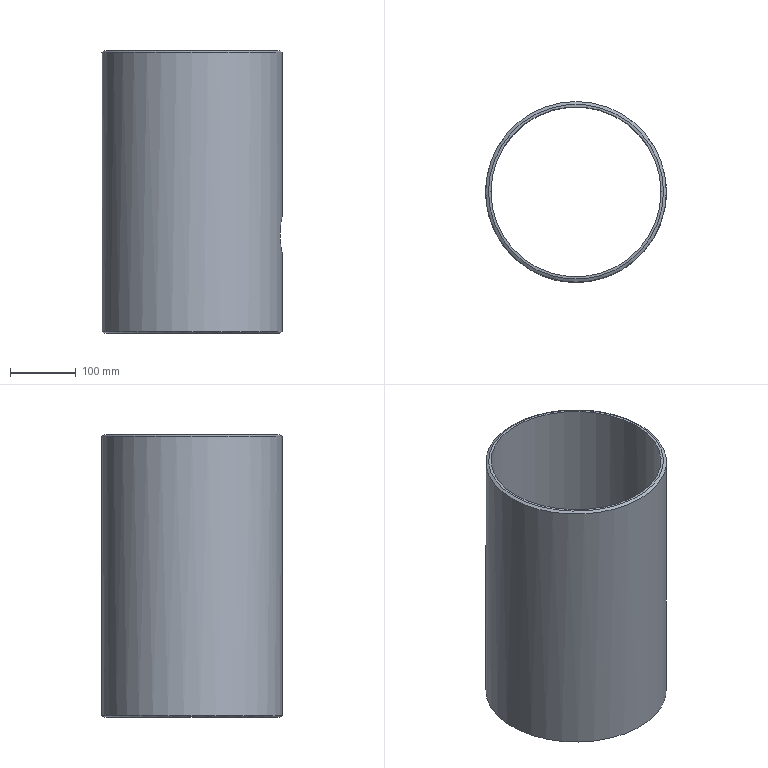Part | NX | features DATUM_CSYS 2, CHAMFER 1, CYLINDER 1, EXTRUDE 1, Resize Face 1, SHELL 1, SKETCH 1 | 1 solid | 7 faces | box 275 x 275 x 430 mm | volume 2853471 mm3 | cylinder 3 | plane 2 | cone 2 | commonest cylinder face diameters 60 x1 259 x1 275 x1
STEP:
#1=CARTESIAN_POINT('',(137.5,0.,2.5));
#2=VERTEX_POINT('',#1);
#3=CARTESIAN_POINT('',(0.,0.,2.5));
#4=DIRECTION('',(0.,0.,1.));
#5=DIRECTION('',(1.,0.,0.));
#6=AXIS2_PLACEMENT_3D('',#3,#4,#5);
#7=CIRCLE('',#6,137.5);
#8=EDGE_CURVE('',#2,#2,#7,.T.);
#9=ORIENTED_EDGE('',*,*,#8,.T.);
#10=EDGE_LOOP('',(#9));
#11=FACE_BOUND('',#10,.T.);
#12=CARTESIAN_POINT('',(-137.5,0.,427.5));
#13=VERTEX_POINT('',#12);
#14=CARTESIAN_POINT('',(0.,0.,427.5));
#15=DIRECTION('',(0.,0.,-1.));
#16=DIRECTION('',(-1.,0.,0.));
#17=AXIS2_PLACEMENT_3D('',#14,#15,#16);
#18=CIRCLE('',#17,137.5);
#19=EDGE_CURVE('',#13,#13,#18,.T.);
#20=ORIENTED_EDGE('',*,*,#19,.T.);
#21=EDGE_LOOP('',(#20));
#22=FACE_BOUND('',#21,.T.);
#23=CARTESIAN_POINT('',(137.5,0.,120.));
#24=VERTEX_POINT('',#23);
#25=CARTESIAN_POINT('',(137.14,11.856,121.591));
#26=CARTESIAN_POINT('',(137.679,-0.009269,119.207));
#27=CARTESIAN_POINT('',(137.143,-11.819,121.58));
#28=CARTESIAN_POINT('',(135.855,-21.765,128.245));
#29=CARTESIAN_POINT('',(134.555,-28.42,138.183));
#30=CARTESIAN_POINT('',(134.004,-30.786,149.979));
#31=CARTESIAN_POINT('',(134.552,-28.435,161.792));
#32=CARTESIAN_POINT('',(135.856,-21.764,171.76));
#33=CARTESIAN_POINT('',(137.143,-11.813,178.423));
#34=CARTESIAN_POINT('',(137.678,-0.01305,180.786));
#35=CARTESIAN_POINT('',(137.145,11.791,178.432));
#36=CARTESIAN_POINT('',(135.859,21.742,171.778));
#37=CARTESIAN_POINT('',(134.556,28.414,161.839));
#38=CARTESIAN_POINT('',(134.004,30.789,150.018));
#39=CARTESIAN_POINT('',(134.553,28.431,138.203));
#40=CARTESIAN_POINT('',(135.854,21.771,128.255));
#41=CARTESIAN_POINT('',(137.14,11.856,121.591));
#42=CARTESIAN_POINT('',(137.679,-0.009269,119.207));
#43=CARTESIAN_POINT('',(137.143,-11.819,121.58));
#44=B_SPLINE_CURVE_WITH_KNOTS('',3,(#25,#26,#27,#28,#29,#30,#31,#32,#33,#34,#35,#36,#37,#38,#39,#40,#41,#42,#43),.UNSPECIFIED.,.T.,.F.,(1,1,1,1,1,1,1,1,1,1,1,1,1,1,1,1,1,1,1,1,1,1,1),(-0.03527,-0.02352,-0.01176,0.,0.01176,0.02352,0.03527,0.04703,0.05879,0.07055,0.08231,0.09406,0.1058,0.1176,0.1293,0.1411,0.1529,0.1646,0.1764,0.1881,0.1999,0.2116,0.2234),.UNSPECIFIED.);
#45=EDGE_CURVE('',#24,#24,#44,.T.);
#46=ORIENTED_EDGE('',*,*,#45,.T.);
#47=EDGE_LOOP('',(#46));
#48=FACE_BOUND('',#47,.T.);
#49=CARTESIAN_POINT('',(0.,0.,0.));
#50=DIRECTION('',(0.,0.,1.));
#51=DIRECTION('',(1.,0.,0.));
#52=AXIS2_PLACEMENT_3D('',#49,#50,#51);
#53=CYLINDRICAL_SURFACE('',#52,137.5);
#54=ADVANCED_FACE('',(#11,#22,#48),#53,.T.);
#55=CARTESIAN_POINT('',(129.5,0.,430.));
#56=VERTEX_POINT('',#55);
#57=CARTESIAN_POINT('',(0.,0.,430.));
#58=DIRECTION('',(0.,0.,1.));
#59=DIRECTION('',(1.,0.,0.));
#60=AXIS2_PLACEMENT_3D('',#57,#58,#59);
#61=CIRCLE('',#60,129.5);
#62=EDGE_CURVE('',#56,#56,#61,.F.);
#63=ORIENTED_EDGE('',*,*,#62,.F.);
#64=EDGE_LOOP('',(#63));
#65=FACE_BOUND('',#64,.T.);
#66=CARTESIAN_POINT('',(-129.5,0.,0.));
#67=VERTEX_POINT('',#66);
#68=CARTESIAN_POINT('',(0.,0.,0.));
#69=DIRECTION('',(0.,0.,-1.));
#70=DIRECTION('',(-1.,0.,0.));
#71=AXIS2_PLACEMENT_3D('',#68,#69,#70);
#72=CIRCLE('',#71,129.5);
#73=EDGE_CURVE('',#67,#67,#72,.F.);
#74=ORIENTED_EDGE('',*,*,#73,.F.);
#75=EDGE_LOOP('',(#74));
#76=FACE_BOUND('',#75,.T.);
#77=CARTESIAN_POINT('',(129.5,0.,120.));
#78=VERTEX_POINT('',#77);
#79=CARTESIAN_POINT('',(129.118,11.859,121.593));
#80=CARTESIAN_POINT('',(129.691,-0.008952,119.206));
#81=CARTESIAN_POINT('',(129.12,-11.823,121.581));
#82=CARTESIAN_POINT('',(127.753,-21.765,128.246));
#83=CARTESIAN_POINT('',(126.369,-28.418,138.179));
#84=CARTESIAN_POINT('',(125.782,-30.787,149.978));
#85=CARTESIAN_POINT('',(126.366,-28.433,161.796));
#86=CARTESIAN_POINT('',(127.754,-21.762,171.761));
#87=CARTESIAN_POINT('',(129.121,-11.817,178.421));
#88=CARTESIAN_POINT('',(129.689,-0.01338,180.787));
#89=CARTESIAN_POINT('',(129.123,11.795,178.431));
#90=CARTESIAN_POINT('',(127.757,21.743,171.777));
#91=CARTESIAN_POINT('',(126.371,28.413,161.842));
#92=CARTESIAN_POINT('',(125.781,30.79,150.017));
#93=CARTESIAN_POINT('',(126.367,28.429,138.198));
#94=CARTESIAN_POINT('',(127.751,21.77,128.255));
#95=CARTESIAN_POINT('',(129.118,11.859,121.593));
#96=CARTESIAN_POINT('',(129.691,-0.008952,119.206));
#97=CARTESIAN_POINT('',(129.12,-11.823,121.581));
#98=B_SPLINE_CURVE_WITH_KNOTS('',3,(#79,#80,#81,#82,#83,#84,#85,#86,#87,#88,#89,#90,#91,#92,#93,#94,#95,#96,#97),.UNSPECIFIED.,.T.,.F.,(1,1,1,1,1,1,1,1,1,1,1,1,1,1,1,1,1,1,1,1,1,1,1),(-0.03529,-0.02353,-0.01176,0.,0.01176,0.02353,0.03529,0.04705,0.05881,0.07058,0.08234,0.0941,0.1059,0.1176,0.1294,0.1412,0.1529,0.1647,0.1764,0.1882,0.2,0.2117,0.2235),.UNSPECIFIED.);
#99=EDGE_CURVE('',#78,#78,#98,.T.);
#100=ORIENTED_EDGE('',*,*,#99,.F.);
#101=EDGE_LOOP('',(#100));
#102=FACE_BOUND('',#101,.T.);
#103=CARTESIAN_POINT('',(0.,0.,0.));
#104=DIRECTION('',(0.,0.,1.));
#105=DIRECTION('',(1.,0.,0.));
#106=AXIS2_PLACEMENT_3D('',#103,#104,#105);
#107=CYLINDRICAL_SURFACE('',#106,129.5);
#108=ADVANCED_FACE('',(#65,#76,#102),#107,.F.);
#109=CARTESIAN_POINT('',(133.17,0.,430.));
#110=VERTEX_POINT('',#109);
#111=CARTESIAN_POINT('',(0.,0.,430.));
#112=DIRECTION('',(0.,0.,1.));
#113=DIRECTION('',(1.,0.,0.));
#114=AXIS2_PLACEMENT_3D('',#111,#112,#113);
#115=CIRCLE('',#114,133.17);
#116=EDGE_CURVE('',#110,#110,#115,.T.);
#117=ORIENTED_EDGE('',*,*,#116,.T.);
#118=EDGE_LOOP('',(#117));
#119=FACE_BOUND('',#118,.T.);
#120=ORIENTED_EDGE('',*,*,#62,.T.);
#121=EDGE_LOOP('',(#120));
#122=FACE_BOUND('',#121,.T.);
#123=CARTESIAN_POINT('',(0.,0.,430.));
#124=DIRECTION('',(0.,0.,1.));
#125=DIRECTION('',(1.,0.,0.));
#126=AXIS2_PLACEMENT_3D('',#123,#124,#125);
#127=PLANE('',#126);
#128=ADVANCED_FACE('',(#119,#122),#127,.T.);
#129=CARTESIAN_POINT('',(-133.17,0.,0.));
#130=VERTEX_POINT('',#129);
#131=CARTESIAN_POINT('',(0.,0.,0.));
#132=DIRECTION('',(0.,0.,-1.));
#133=DIRECTION('',(-1.,0.,0.));
#134=AXIS2_PLACEMENT_3D('',#131,#132,#133);
#135=CIRCLE('',#134,133.17);
#136=EDGE_CURVE('',#130,#130,#135,.T.);
#137=ORIENTED_EDGE('',*,*,#136,.T.);
#138=EDGE_LOOP('',(#137));
#139=FACE_BOUND('',#138,.T.);
#140=ORIENTED_EDGE('',*,*,#73,.T.);
#141=EDGE_LOOP('',(#140));
#142=FACE_BOUND('',#141,.T.);
#143=CARTESIAN_POINT('',(0.,0.,0.));
#144=DIRECTION('',(0.,0.,-1.));
#145=DIRECTION('',(-1.,0.,0.));
#146=AXIS2_PLACEMENT_3D('',#143,#144,#145);
#147=PLANE('',#146);
#148=ADVANCED_FACE('',(#139,#142),#147,.T.);
#149=ORIENTED_EDGE('',*,*,#116,.F.);
#150=EDGE_LOOP('',(#149));
#151=FACE_BOUND('',#150,.T.);
#152=ORIENTED_EDGE('',*,*,#19,.F.);
#153=EDGE_LOOP('',(#152));
#154=FACE_BOUND('',#153,.T.);
#155=CARTESIAN_POINT('',(0.,0.,427.5));
#156=DIRECTION('',(0.,0.,-1.));
#157=DIRECTION('',(-1.,0.,0.));
#158=AXIS2_PLACEMENT_3D('',#155,#156,#157);
#159=CONICAL_SURFACE('',#158,137.5,1.047);
#160=ADVANCED_FACE('',(#151,#154),#159,.T.);
#161=ORIENTED_EDGE('',*,*,#136,.F.);
#162=EDGE_LOOP('',(#161));
#163=FACE_BOUND('',#162,.T.);
#164=ORIENTED_EDGE('',*,*,#8,.F.);
#165=EDGE_LOOP('',(#164));
#166=FACE_BOUND('',#165,.T.);
#167=CARTESIAN_POINT('',(0.,0.,2.5));
#168=DIRECTION('',(0.,0.,1.));
#169=DIRECTION('',(1.,0.,0.));
#170=AXIS2_PLACEMENT_3D('',#167,#168,#169);
#171=CONICAL_SURFACE('',#170,137.5,1.047);
#172=ADVANCED_FACE('',(#163,#166),#171,.T.);
#173=ORIENTED_EDGE('',*,*,#45,.F.);
#174=EDGE_LOOP('',(#173));
#175=FACE_BOUND('',#174,.T.);
#176=ORIENTED_EDGE('',*,*,#99,.T.);
#177=EDGE_LOOP('',(#176));
#178=FACE_BOUND('',#177,.T.);
#179=CARTESIAN_POINT('',(720.,0.,150.));
#180=DIRECTION('',(-1.,0.,0.));
#181=DIRECTION('',(0.,0.,1.));
#182=AXIS2_PLACEMENT_3D('',#179,#180,#181);
#183=CYLINDRICAL_SURFACE('',#182,30.);
#184=ADVANCED_FACE('',(#175,#178),#183,.F.);
#185=CLOSED_SHELL('',(#54,#108,#128,#148,#160,#172,#184));
#186=MANIFOLD_SOLID_BREP('',#185);
#187=(LENGTH_UNIT()NAMED_UNIT(*)SI_UNIT(.MILLI.,.METRE.));
#188=UNCERTAINTY_MEASURE_WITH_UNIT(LENGTH_MEASURE(0.0508),#187,'','');
#189=(NAMED_UNIT(*)PLANE_ANGLE_UNIT()SI_UNIT($,.RADIAN.));
#190=(NAMED_UNIT(*)SI_UNIT($,.STERADIAN.)SOLID_ANGLE_UNIT());
#191=(GEOMETRIC_REPRESENTATION_CONTEXT(3)GLOBAL_UNCERTAINTY_ASSIGNED_CONTEXT((#188))GLOBAL_UNIT_ASSIGNED_CONTEXT((#187,#189,#190))REPRESENTATION_CONTEXT('',''));
#192=ADVANCED_BREP_SHAPE_REPRESENTATION('',(#186),#191);